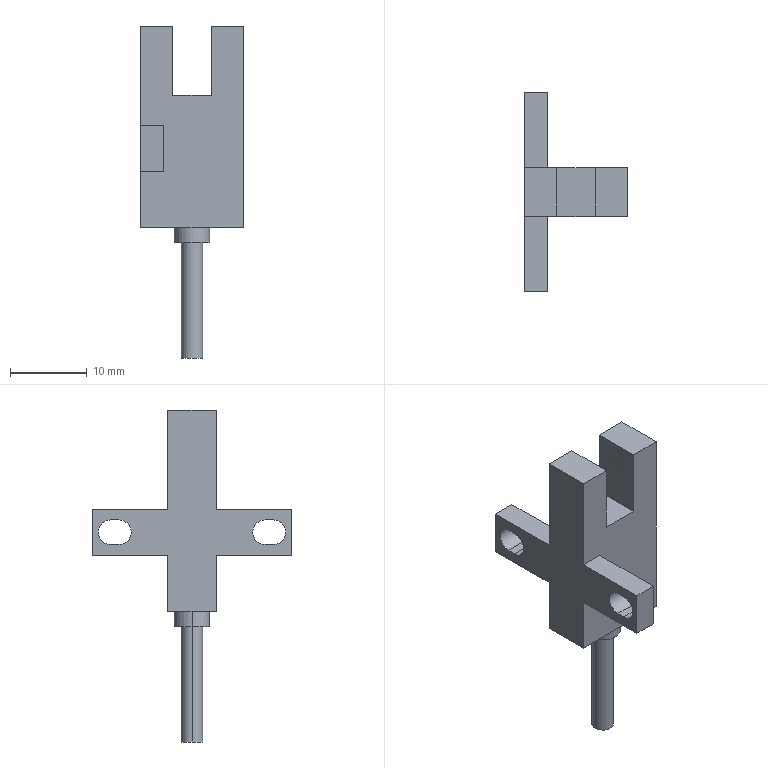Part | NX | features BREP 1 | 1 solid | 47 faces | box 13.4 x 26 x 43.2 mm | volume 2353 mm3 | plane 39 | cylinder 8 | commonest cylinder face diameters 3.2 x4 2.8 x2 4.6 x2
STEP:
#1=CARTESIAN_POINT('',(-1.4,0.,-2.));
#2=VERTEX_POINT('',#1);
#3=CARTESIAN_POINT('',(1.4,0.,-2.));
#4=VERTEX_POINT('',#3);
#5=CARTESIAN_POINT('',(0.,0.,-2.));
#6=DIRECTION('',(0.,0.,-1.));
#7=DIRECTION('',(-1.,0.,0.));
#8=AXIS2_PLACEMENT_3D('',#5,#6,#7);
#9=CIRCLE('',#8,1.4);
#10=EDGE_CURVE('',#2,#4,#9,.T.);
#11=ORIENTED_EDGE('',*,*,#10,.F.);
#12=CARTESIAN_POINT('',(0.,0.,-2.));
#13=DIRECTION('',(0.,0.,-1.));
#14=DIRECTION('',(-1.,0.,0.));
#15=AXIS2_PLACEMENT_3D('',#12,#13,#14);
#16=CIRCLE('',#15,1.4);
#17=EDGE_CURVE('',#4,#2,#16,.T.);
#18=ORIENTED_EDGE('',*,*,#17,.F.);
#19=EDGE_LOOP('',(#11,#18));
#20=FACE_BOUND('',#19,.T.);
#21=CARTESIAN_POINT('',(-2.3,0.,-2.));
#22=VERTEX_POINT('',#21);
#23=CARTESIAN_POINT('',(2.3,0.,-2.));
#24=VERTEX_POINT('',#23);
#25=CARTESIAN_POINT('',(0.,0.,-2.));
#26=DIRECTION('',(0.,0.,-1.));
#27=DIRECTION('',(-1.,0.,0.));
#28=AXIS2_PLACEMENT_3D('',#25,#26,#27);
#29=CIRCLE('',#28,2.3);
#30=EDGE_CURVE('',#22,#24,#29,.T.);
#31=ORIENTED_EDGE('',*,*,#30,.T.);
#32=CARTESIAN_POINT('',(0.,0.,-2.));
#33=DIRECTION('',(0.,0.,-1.));
#34=DIRECTION('',(-1.,0.,0.));
#35=AXIS2_PLACEMENT_3D('',#32,#33,#34);
#36=CIRCLE('',#35,2.3);
#37=EDGE_CURVE('',#24,#22,#36,.T.);
#38=ORIENTED_EDGE('',*,*,#37,.T.);
#39=EDGE_LOOP('',(#31,#38));
#40=FACE_BOUND('',#39,.T.);
#41=CARTESIAN_POINT('',(1.4,0.,-2.));
#42=DIRECTION('',(0.,0.,-1.));
#43=DIRECTION('',(-1.,0.,0.));
#44=AXIS2_PLACEMENT_3D('',#41,#42,#43);
#45=PLANE('',#44);
#46=ADVANCED_FACE('',(#20,#40),#45,.T.);
#47=CARTESIAN_POINT('',(1.4,0.,-17.));
#48=VERTEX_POINT('',#47);
#49=CARTESIAN_POINT('',(1.4,0.,0.));
#50=DIRECTION('',(0.,0.,-1.));
#51=VECTOR('',#50,1000.);
#52=LINE('',#49,#51);
#53=EDGE_CURVE('',#4,#48,#52,.T.);
#54=ORIENTED_EDGE('',*,*,#53,.F.);
#55=ORIENTED_EDGE('',*,*,#17,.T.);
#56=CARTESIAN_POINT('',(-1.4,0.,-17.));
#57=VERTEX_POINT('',#56);
#58=CARTESIAN_POINT('',(-1.4,0.,0.));
#59=DIRECTION('',(0.,0.,-1.));
#60=VECTOR('',#59,1000.);
#61=LINE('',#58,#60);
#62=EDGE_CURVE('',#2,#57,#61,.T.);
#63=ORIENTED_EDGE('',*,*,#62,.T.);
#64=CARTESIAN_POINT('',(0.,0.,-17.));
#65=DIRECTION('',(0.,0.,-1.));
#66=DIRECTION('',(-1.,0.,0.));
#67=AXIS2_PLACEMENT_3D('',#64,#65,#66);
#68=CIRCLE('',#67,1.4);
#69=EDGE_CURVE('',#48,#57,#68,.T.);
#70=ORIENTED_EDGE('',*,*,#69,.F.);
#71=EDGE_LOOP('',(#54,#55,#63,#70));
#72=FACE_BOUND('',#71,.T.);
#73=CARTESIAN_POINT('',(0.,0.,0.));
#74=DIRECTION('',(0.,0.,-1.));
#75=DIRECTION('',(-1.,0.,0.));
#76=AXIS2_PLACEMENT_3D('',#73,#74,#75);
#77=CYLINDRICAL_SURFACE('',#76,1.4);
#78=ADVANCED_FACE('',(#72),#77,.T.);
#79=CARTESIAN_POINT('',(0.,0.,-17.));
#80=DIRECTION('',(0.,0.,-1.));
#81=DIRECTION('',(-1.,0.,0.));
#82=AXIS2_PLACEMENT_3D('',#79,#80,#81);
#83=CIRCLE('',#82,1.4);
#84=EDGE_CURVE('',#57,#48,#83,.T.);
#85=ORIENTED_EDGE('',*,*,#84,.T.);
#86=ORIENTED_EDGE('',*,*,#69,.T.);
#87=EDGE_LOOP('',(#85,#86));
#88=FACE_BOUND('',#87,.T.);
#89=CARTESIAN_POINT('',(0.,0.,-17.));
#90=DIRECTION('',(0.,0.,-1.));
#91=DIRECTION('',(-1.,0.,0.));
#92=AXIS2_PLACEMENT_3D('',#89,#90,#91);
#93=PLANE('',#92);
#94=ADVANCED_FACE('',(#88),#93,.T.);
#95=CARTESIAN_POINT('',(2.3,0.,0.));
#96=VERTEX_POINT('',#95);
#97=CARTESIAN_POINT('',(2.3,0.,0.));
#98=DIRECTION('',(0.,0.,-1.));
#99=VECTOR('',#98,1000.);
#100=LINE('',#97,#99);
#101=EDGE_CURVE('',#96,#24,#100,.T.);
#102=ORIENTED_EDGE('',*,*,#101,.F.);
#103=CARTESIAN_POINT('',(-2.3,0.,0.));
#104=VERTEX_POINT('',#103);
#105=CARTESIAN_POINT('',(0.,0.,0.));
#106=DIRECTION('',(0.,0.,-1.));
#107=DIRECTION('',(-1.,0.,0.));
#108=AXIS2_PLACEMENT_3D('',#105,#106,#107);
#109=CIRCLE('',#108,2.3);
#110=EDGE_CURVE('',#96,#104,#109,.T.);
#111=ORIENTED_EDGE('',*,*,#110,.T.);
#112=CARTESIAN_POINT('',(-2.3,0.,0.));
#113=DIRECTION('',(0.,0.,-1.));
#114=VECTOR('',#113,1000.);
#115=LINE('',#112,#114);
#116=EDGE_CURVE('',#104,#22,#115,.T.);
#117=ORIENTED_EDGE('',*,*,#116,.T.);
#118=ORIENTED_EDGE('',*,*,#37,.F.);
#119=EDGE_LOOP('',(#102,#111,#117,#118));
#120=FACE_BOUND('',#119,.T.);
#121=CARTESIAN_POINT('',(0.,0.,0.));
#122=DIRECTION('',(0.,0.,-1.));
#123=DIRECTION('',(-1.,0.,0.));
#124=AXIS2_PLACEMENT_3D('',#121,#122,#123);
#125=CYLINDRICAL_SURFACE('',#124,2.3);
#126=ADVANCED_FACE('',(#120),#125,.T.);
#127=CARTESIAN_POINT('',(2.55,-0.4,22.3));
#128=VERTEX_POINT('',#127);
#129=CARTESIAN_POINT('',(2.55,-0.4,24.3));
#130=VERTEX_POINT('',#129);
#131=CARTESIAN_POINT('',(2.55,-0.4,22.3));
#132=DIRECTION('',(0.,0.,1.));
#133=VECTOR('',#132,1000.);
#134=LINE('',#131,#133);
#135=EDGE_CURVE('',#128,#130,#134,.T.);
#136=ORIENTED_EDGE('',*,*,#135,.T.);
#137=CARTESIAN_POINT('',(2.55,0.4,24.3));
#138=VERTEX_POINT('',#137);
#139=CARTESIAN_POINT('',(2.55,-0.4,24.3));
#140=DIRECTION('',(0.,1.,0.));
#141=VECTOR('',#140,1000.);
#142=LINE('',#139,#141);
#143=EDGE_CURVE('',#130,#138,#142,.T.);
#144=ORIENTED_EDGE('',*,*,#143,.T.);
#145=CARTESIAN_POINT('',(2.55,0.4,22.3));
#146=VERTEX_POINT('',#145);
#147=CARTESIAN_POINT('',(2.55,0.4,24.3));
#148=DIRECTION('',(0.,0.,-1.));
#149=VECTOR('',#148,1000.);
#150=LINE('',#147,#149);
#151=EDGE_CURVE('',#138,#146,#150,.T.);
#152=ORIENTED_EDGE('',*,*,#151,.T.);
#153=CARTESIAN_POINT('',(2.55,0.4,22.3));
#154=DIRECTION('',(0.,-1.,0.));
#155=VECTOR('',#154,1000.);
#156=LINE('',#153,#155);
#157=EDGE_CURVE('',#146,#128,#156,.T.);
#158=ORIENTED_EDGE('',*,*,#157,.T.);
#159=EDGE_LOOP('',(#136,#144,#152,#158));
#160=FACE_BOUND('',#159,.T.);
#161=CARTESIAN_POINT('',(2.55,0.,0.));
#162=DIRECTION('',(-1.,0.,0.));
#163=DIRECTION('',(0.,0.,1.));
#164=AXIS2_PLACEMENT_3D('',#161,#162,#163);
#165=PLANE('',#164);
#166=ADVANCED_FACE('',(#160),#165,.T.);
#167=CARTESIAN_POINT('',(2.5,-0.4,24.3));
#168=VERTEX_POINT('',#167);
#169=CARTESIAN_POINT('',(2.5,0.4,24.3));
#170=VERTEX_POINT('',#169);
#171=CARTESIAN_POINT('',(2.5,-0.4,24.3));
#172=DIRECTION('',(0.,1.,0.));
#173=VECTOR('',#172,1000.);
#174=LINE('',#171,#173);
#175=EDGE_CURVE('',#168,#170,#174,.T.);
#176=ORIENTED_EDGE('',*,*,#175,.T.);
#177=CARTESIAN_POINT('',(2.55,0.4,24.3));
#178=DIRECTION('',(-1.,0.,0.));
#179=VECTOR('',#178,1000.);
#180=LINE('',#177,#179);
#181=EDGE_CURVE('',#138,#170,#180,.T.);
#182=ORIENTED_EDGE('',*,*,#181,.F.);
#183=ORIENTED_EDGE('',*,*,#143,.F.);
#184=CARTESIAN_POINT('',(2.55,-0.4,24.3));
#185=DIRECTION('',(-1.,0.,0.));
#186=VECTOR('',#185,1000.);
#187=LINE('',#184,#186);
#188=EDGE_CURVE('',#130,#168,#187,.T.);
#189=ORIENTED_EDGE('',*,*,#188,.T.);
#190=EDGE_LOOP('',(#176,#182,#183,#189));
#191=FACE_BOUND('',#190,.T.);
#192=CARTESIAN_POINT('',(2.55,-0.4,24.3));
#193=DIRECTION('',(0.,0.,1.));
#194=DIRECTION('',(1.,0.,0.));
#195=AXIS2_PLACEMENT_3D('',#192,#193,#194);
#196=PLANE('',#195);
#197=ADVANCED_FACE('',(#191),#196,.F.);
#198=CARTESIAN_POINT('',(2.5,0.4,22.3));
#199=VERTEX_POINT('',#198);
#200=CARTESIAN_POINT('',(2.5,0.4,24.3));
#201=DIRECTION('',(0.,0.,-1.));
#202=VECTOR('',#201,1000.);
#203=LINE('',#200,#202);
#204=EDGE_CURVE('',#170,#199,#203,.T.);
#205=ORIENTED_EDGE('',*,*,#204,.T.);
#206=CARTESIAN_POINT('',(2.55,0.4,22.3));
#207=DIRECTION('',(-1.,0.,0.));
#208=VECTOR('',#207,1000.);
#209=LINE('',#206,#208);
#210=EDGE_CURVE('',#146,#199,#209,.T.);
#211=ORIENTED_EDGE('',*,*,#210,.F.);
#212=ORIENTED_EDGE('',*,*,#151,.F.);
#213=ORIENTED_EDGE('',*,*,#181,.T.);
#214=EDGE_LOOP('',(#205,#211,#212,#213));
#215=FACE_BOUND('',#214,.T.);
#216=CARTESIAN_POINT('',(2.55,0.4,24.3));
#217=DIRECTION('',(0.,1.,0.));
#218=DIRECTION('',(0.,0.,1.));
#219=AXIS2_PLACEMENT_3D('',#216,#217,#218);
#220=PLANE('',#219);
#221=ADVANCED_FACE('',(#215),#220,.F.);
#222=CARTESIAN_POINT('',(2.5,-0.4,22.3));
#223=VERTEX_POINT('',#222);
#224=CARTESIAN_POINT('',(2.5,0.4,22.3));
#225=DIRECTION('',(0.,-1.,0.));
#226=VECTOR('',#225,1000.);
#227=LINE('',#224,#226);
#228=EDGE_CURVE('',#199,#223,#227,.T.);
#229=ORIENTED_EDGE('',*,*,#228,.T.);
#230=CARTESIAN_POINT('',(2.55,-0.4,22.3));
#231=DIRECTION('',(-1.,0.,0.));
#232=VECTOR('',#231,1000.);
#233=LINE('',#230,#232);
#234=EDGE_CURVE('',#128,#223,#233,.T.);
#235=ORIENTED_EDGE('',*,*,#234,.F.);
#236=ORIENTED_EDGE('',*,*,#157,.F.);
#237=ORIENTED_EDGE('',*,*,#210,.T.);
#238=EDGE_LOOP('',(#229,#235,#236,#237));
#239=FACE_BOUND('',#238,.T.);
#240=CARTESIAN_POINT('',(2.55,0.4,22.3));
#241=DIRECTION('',(0.,0.,-1.));
#242=DIRECTION('',(-1.,0.,0.));
#243=AXIS2_PLACEMENT_3D('',#240,#241,#242);
#244=PLANE('',#243);
#245=ADVANCED_FACE('',(#239),#244,.F.);
#246=CARTESIAN_POINT('',(2.5,-0.4,22.3));
#247=DIRECTION('',(0.,0.,1.));
#248=VECTOR('',#247,1000.);
#249=LINE('',#246,#248);
#250=EDGE_CURVE('',#223,#168,#249,.T.);
#251=ORIENTED_EDGE('',*,*,#250,.T.);
#252=ORIENTED_EDGE('',*,*,#188,.F.);
#253=ORIENTED_EDGE('',*,*,#135,.F.);
#254=ORIENTED_EDGE('',*,*,#234,.T.);
#255=EDGE_LOOP('',(#251,#252,#253,#254));
#256=FACE_BOUND('',#255,.T.);
#257=CARTESIAN_POINT('',(2.55,-0.4,22.3));
#258=DIRECTION('',(0.,-1.,0.));
#259=DIRECTION('',(0.,0.,-1.));
#260=AXIS2_PLACEMENT_3D('',#257,#258,#259);
#261=PLANE('',#260);
#262=ADVANCED_FACE('',(#256),#261,.F.);
#263=CARTESIAN_POINT('',(-2.55,-0.4,22.3));
#264=VERTEX_POINT('',#263);
#265=CARTESIAN_POINT('',(-2.55,0.4,22.3));
#266=VERTEX_POINT('',#265);
#267=CARTESIAN_POINT('',(-2.55,-0.4,22.3));
#268=DIRECTION('',(0.,1.,0.));
#269=VECTOR('',#268,1000.);
#270=LINE('',#267,#269);
#271=EDGE_CURVE('',#264,#266,#270,.T.);
#272=ORIENTED_EDGE('',*,*,#271,.T.);
#273=CARTESIAN_POINT('',(-2.55,0.4,24.3));
#274=VERTEX_POINT('',#273);
#275=CARTESIAN_POINT('',(-2.55,0.4,22.3));
#276=DIRECTION('',(0.,0.,1.));
#277=VECTOR('',#276,1000.);
#278=LINE('',#275,#277);
#279=EDGE_CURVE('',#266,#274,#278,.T.);
#280=ORIENTED_EDGE('',*,*,#279,.T.);
#281=CARTESIAN_POINT('',(-2.55,-0.4,24.3));
#282=VERTEX_POINT('',#281);
#283=CARTESIAN_POINT('',(-2.55,0.4,24.3));
#284=DIRECTION('',(0.,-1.,0.));
#285=VECTOR('',#284,1000.);
#286=LINE('',#283,#285);
#287=EDGE_CURVE('',#274,#282,#286,.T.);
#288=ORIENTED_EDGE('',*,*,#287,.T.);
#289=CARTESIAN_POINT('',(-2.55,-0.4,24.3));
#290=DIRECTION('',(0.,0.,-1.));
#291=VECTOR('',#290,1000.);
#292=LINE('',#289,#291);
#293=EDGE_CURVE('',#282,#264,#292,.T.);
#294=ORIENTED_EDGE('',*,*,#293,.T.);
#295=EDGE_LOOP('',(#272,#280,#288,#294));
#296=FACE_BOUND('',#295,.T.);
#297=CARTESIAN_POINT('',(-2.55,0.,0.));
#298=DIRECTION('',(1.,0.,0.));
#299=DIRECTION('',(0.,0.,-1.));
#300=AXIS2_PLACEMENT_3D('',#297,#298,#299);
#301=PLANE('',#300);
#302=ADVANCED_FACE('',(#296),#301,.T.);
#303=CARTESIAN_POINT('',(-2.5,0.4,22.3));
#304=VERTEX_POINT('',#303);
#305=CARTESIAN_POINT('',(-2.5,0.4,24.3));
#306=VERTEX_POINT('',#305);
#307=CARTESIAN_POINT('',(-2.5,0.4,22.3));
#308=DIRECTION('',(0.,0.,1.));
#309=VECTOR('',#308,1000.);
#310=LINE('',#307,#309);
#311=EDGE_CURVE('',#304,#306,#310,.T.);
#312=ORIENTED_EDGE('',*,*,#311,.T.);
#313=CARTESIAN_POINT('',(-2.55,0.4,24.3));
#314=DIRECTION('',(1.,0.,0.));
#315=VECTOR('',#314,1000.);
#316=LINE('',#313,#315);
#317=EDGE_CURVE('',#274,#306,#316,.T.);
#318=ORIENTED_EDGE('',*,*,#317,.F.);
#319=ORIENTED_EDGE('',*,*,#279,.F.);
#320=CARTESIAN_POINT('',(-2.55,0.4,22.3));
#321=DIRECTION('',(1.,0.,0.));
#322=VECTOR('',#321,1000.);
#323=LINE('',#320,#322);
#324=EDGE_CURVE('',#266,#304,#323,.T.);
#325=ORIENTED_EDGE('',*,*,#324,.T.);
#326=EDGE_LOOP('',(#312,#318,#319,#325));
#327=FACE_BOUND('',#326,.T.);
#328=CARTESIAN_POINT('',(-2.55,0.4,22.3));
#329=DIRECTION('',(0.,1.,0.));
#330=DIRECTION('',(0.,0.,1.));
#331=AXIS2_PLACEMENT_3D('',#328,#329,#330);
#332=PLANE('',#331);
#333=ADVANCED_FACE('',(#327),#332,.F.);
#334=CARTESIAN_POINT('',(-2.5,-0.4,24.3));
#335=VERTEX_POINT('',#334);
#336=CARTESIAN_POINT('',(-2.5,0.4,24.3));
#337=DIRECTION('',(0.,-1.,0.));
#338=VECTOR('',#337,1000.);
#339=LINE('',#336,#338);
#340=EDGE_CURVE('',#306,#335,#339,.T.);
#341=ORIENTED_EDGE('',*,*,#340,.T.);
#342=CARTESIAN_POINT('',(-2.55,-0.4,24.3));
#343=DIRECTION('',(1.,0.,0.));
#344=VECTOR('',#343,1000.);
#345=LINE('',#342,#344);
#346=EDGE_CURVE('',#282,#335,#345,.T.);
#347=ORIENTED_EDGE('',*,*,#346,.F.);
#348=ORIENTED_EDGE('',*,*,#287,.F.);
#349=ORIENTED_EDGE('',*,*,#317,.T.);
#350=EDGE_LOOP('',(#341,#347,#348,#349));
#351=FACE_BOUND('',#350,.T.);
#352=CARTESIAN_POINT('',(-2.55,0.4,24.3));
#353=DIRECTION('',(0.,0.,1.));
#354=DIRECTION('',(1.,0.,0.));
#355=AXIS2_PLACEMENT_3D('',#352,#353,#354);
#356=PLANE('',#355);
#357=ADVANCED_FACE('',(#351),#356,.F.);
#358=CARTESIAN_POINT('',(-2.5,-0.4,22.3));
#359=VERTEX_POINT('',#358);
#360=CARTESIAN_POINT('',(-2.5,-0.4,24.3));
#361=DIRECTION('',(0.,0.,-1.));
#362=VECTOR('',#361,1000.);
#363=LINE('',#360,#362);
#364=EDGE_CURVE('',#335,#359,#363,.T.);
#365=ORIENTED_EDGE('',*,*,#364,.T.);
#366=CARTESIAN_POINT('',(-2.55,-0.4,22.3));
#367=DIRECTION('',(1.,0.,0.));
#368=VECTOR('',#367,1000.);
#369=LINE('',#366,#368);
#370=EDGE_CURVE('',#264,#359,#369,.T.);
#371=ORIENTED_EDGE('',*,*,#370,.F.);
#372=ORIENTED_EDGE('',*,*,#293,.F.);
#373=ORIENTED_EDGE('',*,*,#346,.T.);
#374=EDGE_LOOP('',(#365,#371,#372,#373));
#375=FACE_BOUND('',#374,.T.);
#376=CARTESIAN_POINT('',(-2.55,-0.4,24.3));
#377=DIRECTION('',(0.,-1.,0.));
#378=DIRECTION('',(0.,0.,-1.));
#379=AXIS2_PLACEMENT_3D('',#376,#377,#378);
#380=PLANE('',#379);
#381=ADVANCED_FACE('',(#375),#380,.F.);
#382=CARTESIAN_POINT('',(-2.5,-0.4,22.3));
#383=DIRECTION('',(0.,1.,0.));
#384=VECTOR('',#383,1000.);
#385=LINE('',#382,#384);
#386=EDGE_CURVE('',#359,#304,#385,.T.);
#387=ORIENTED_EDGE('',*,*,#386,.T.);
#388=ORIENTED_EDGE('',*,*,#324,.F.);
#389=ORIENTED_EDGE('',*,*,#271,.F.);
#390=ORIENTED_EDGE('',*,*,#370,.T.);
#391=EDGE_LOOP('',(#387,#388,#389,#390));
#392=FACE_BOUND('',#391,.T.);
#393=CARTESIAN_POINT('',(-2.55,-0.4,22.3));
#394=DIRECTION('',(0.,0.,-1.));
#395=DIRECTION('',(-1.,0.,0.));
#396=AXIS2_PLACEMENT_3D('',#393,#394,#395);
#397=PLANE('',#396);
#398=ADVANCED_FACE('',(#392),#397,.F.);
#399=CARTESIAN_POINT('',(3.,3.125,11.3));
#400=VERTEX_POINT('',#399);
#401=CARTESIAN_POINT('',(3.,3.125,8.8));
#402=VERTEX_POINT('',#401);
#403=CARTESIAN_POINT('',(3.,3.125,11.3));
#404=DIRECTION('',(0.,0.,-1.));
#405=VECTOR('',#404,1000.);
#406=LINE('',#403,#405);
#407=EDGE_CURVE('',#400,#402,#406,.T.);
#408=ORIENTED_EDGE('',*,*,#407,.T.);
#409=CARTESIAN_POINT('',(0.,3.125,8.8));
#410=VERTEX_POINT('',#409);
#411=CARTESIAN_POINT('',(3.,3.125,8.8));
#412=DIRECTION('',(-1.,0.,0.));
#413=VECTOR('',#412,1000.);
#414=LINE('',#411,#413);
#415=EDGE_CURVE('',#402,#410,#414,.T.);
#416=ORIENTED_EDGE('',*,*,#415,.T.);
#417=CARTESIAN_POINT('',(0.,3.125,11.3));
#418=VERTEX_POINT('',#417);
#419=CARTESIAN_POINT('',(0.,3.125,8.8));
#420=DIRECTION('',(0.,0.,1.));
#421=VECTOR('',#420,1000.);
#422=LINE('',#419,#421);
#423=EDGE_CURVE('',#410,#418,#422,.T.);
#424=ORIENTED_EDGE('',*,*,#423,.T.);
#425=CARTESIAN_POINT('',(0.,3.125,11.3));
#426=DIRECTION('',(1.,0.,0.));
#427=VECTOR('',#426,1000.);
#428=LINE('',#425,#427);
#429=EDGE_CURVE('',#418,#400,#428,.T.);
#430=ORIENTED_EDGE('',*,*,#429,.T.);
#431=EDGE_LOOP('',(#408,#416,#424,#430));
#432=FACE_BOUND('',#431,.T.);
#433=CARTESIAN_POINT('',(0.,3.125,0.));
#434=DIRECTION('',(0.,1.,0.));
#435=DIRECTION('',(0.,0.,1.));
#436=AXIS2_PLACEMENT_3D('',#433,#434,#435);
#437=PLANE('',#436);
#438=ADVANCED_FACE('',(#432),#437,.T.);
#439=CARTESIAN_POINT('',(3.,3.175,8.8));
#440=VERTEX_POINT('',#439);
#441=CARTESIAN_POINT('',(0.,3.175,8.8));
#442=VERTEX_POINT('',#441);
#443=CARTESIAN_POINT('',(3.,3.175,8.8));
#444=DIRECTION('',(-1.,0.,0.));
#445=VECTOR('',#444,1000.);
#446=LINE('',#443,#445);
#447=EDGE_CURVE('',#440,#442,#446,.T.);
#448=ORIENTED_EDGE('',*,*,#447,.T.);
#449=CARTESIAN_POINT('',(0.,3.125,8.8));
#450=DIRECTION('',(0.,1.,0.));
#451=VECTOR('',#450,1000.);
#452=LINE('',#449,#451);
#453=EDGE_CURVE('',#410,#442,#452,.T.);
#454=ORIENTED_EDGE('',*,*,#453,.F.);
#455=ORIENTED_EDGE('',*,*,#415,.F.);
#456=CARTESIAN_POINT('',(3.,3.125,8.8));
#457=DIRECTION('',(0.,1.,0.));
#458=VECTOR('',#457,1000.);
#459=LINE('',#456,#458);
#460=EDGE_CURVE('',#402,#440,#459,.T.);
#461=ORIENTED_EDGE('',*,*,#460,.T.);
#462=EDGE_LOOP('',(#448,#454,#455,#461));
#463=FACE_BOUND('',#462,.T.);
#464=CARTESIAN_POINT('',(3.,3.125,8.8));
#465=DIRECTION('',(0.,0.,-1.));
#466=DIRECTION('',(-1.,0.,0.));
#467=AXIS2_PLACEMENT_3D('',#464,#465,#466);
#468=PLANE('',#467);
#469=ADVANCED_FACE('',(#463),#468,.F.);
#470=CARTESIAN_POINT('',(0.,3.175,11.3));
#471=VERTEX_POINT('',#470);
#472=CARTESIAN_POINT('',(0.,3.175,8.8));
#473=DIRECTION('',(0.,0.,1.));
#474=VECTOR('',#473,1000.);
#475=LINE('',#472,#474);
#476=EDGE_CURVE('',#442,#471,#475,.T.);
#477=ORIENTED_EDGE('',*,*,#476,.T.);
#478=CARTESIAN_POINT('',(0.,3.125,11.3));
#479=DIRECTION('',(0.,1.,0.));
#480=VECTOR('',#479,1000.);
#481=LINE('',#478,#480);
#482=EDGE_CURVE('',#418,#471,#481,.T.);
#483=ORIENTED_EDGE('',*,*,#482,.F.);
#484=ORIENTED_EDGE('',*,*,#423,.F.);
#485=ORIENTED_EDGE('',*,*,#453,.T.);
#486=EDGE_LOOP('',(#477,#483,#484,#485));
#487=FACE_BOUND('',#486,.T.);
#488=CARTESIAN_POINT('',(0.,3.125,8.8));
#489=DIRECTION('',(-1.,0.,0.));
#490=DIRECTION('',(0.,0.,1.));
#491=AXIS2_PLACEMENT_3D('',#488,#489,#490);
#492=PLANE('',#491);
#493=ADVANCED_FACE('',(#487),#492,.F.);
#494=CARTESIAN_POINT('',(3.,3.175,11.3));
#495=VERTEX_POINT('',#494);
#496=CARTESIAN_POINT('',(0.,3.175,11.3));
#497=DIRECTION('',(1.,0.,0.));
#498=VECTOR('',#497,1000.);
#499=LINE('',#496,#498);
#500=EDGE_CURVE('',#471,#495,#499,.T.);
#501=ORIENTED_EDGE('',*,*,#500,.T.);
#502=CARTESIAN_POINT('',(3.,3.125,11.3));
#503=DIRECTION('',(0.,1.,0.));
#504=VECTOR('',#503,1000.);
#505=LINE('',#502,#504);
#506=EDGE_CURVE('',#400,#495,#505,.T.);
#507=ORIENTED_EDGE('',*,*,#506,.F.);
#508=ORIENTED_EDGE('',*,*,#429,.F.);
#509=ORIENTED_EDGE('',*,*,#482,.T.);
#510=EDGE_LOOP('',(#501,#507,#508,#509));
#511=FACE_BOUND('',#510,.T.);
#512=CARTESIAN_POINT('',(0.,3.125,11.3));
#513=DIRECTION('',(0.,0.,1.));
#514=DIRECTION('',(1.,0.,0.));
#515=AXIS2_PLACEMENT_3D('',#512,#513,#514);
#516=PLANE('',#515);
#517=ADVANCED_FACE('',(#511),#516,.F.);
#518=CARTESIAN_POINT('',(3.,3.175,11.3));
#519=DIRECTION('',(0.,0.,-1.));
#520=VECTOR('',#519,1000.);
#521=LINE('',#518,#520);
#522=EDGE_CURVE('',#495,#440,#521,.T.);
#523=ORIENTED_EDGE('',*,*,#522,.T.);
#524=ORIENTED_EDGE('',*,*,#460,.F.);
#525=ORIENTED_EDGE('',*,*,#407,.F.);
#526=ORIENTED_EDGE('',*,*,#506,.T.);
#527=EDGE_LOOP('',(#523,#524,#525,#526));
#528=FACE_BOUND('',#527,.T.);
#529=CARTESIAN_POINT('',(3.,3.125,11.3));
#530=DIRECTION('',(1.,0.,0.));
#531=DIRECTION('',(0.,0.,-1.));
#532=AXIS2_PLACEMENT_3D('',#529,#530,#531);
#533=PLANE('',#532);
#534=ADVANCED_FACE('',(#528),#533,.F.);
#535=CARTESIAN_POINT('',(-3.7,9.5,11.9));
#536=VERTEX_POINT('',#535);
#537=CARTESIAN_POINT('',(-6.7,9.5,11.9));
#538=VERTEX_POINT('',#537);
#539=CARTESIAN_POINT('',(6.7,9.5,11.9));
#540=DIRECTION('',(-1.,0.,0.));
#541=VECTOR('',#540,1000.);
#542=LINE('',#539,#541);
#543=EDGE_CURVE('',#536,#538,#542,.T.);
#544=ORIENTED_EDGE('',*,*,#543,.T.);
#545=CARTESIAN_POINT('',(-6.7,10.6,11.9));
#546=VERTEX_POINT('',#545);
#547=CARTESIAN_POINT('',(-6.7,9.5,11.9));
#548=DIRECTION('',(0.,1.,0.));
#549=VECTOR('',#548,1000.);
#550=LINE('',#547,#549);
#551=EDGE_CURVE('',#538,#546,#550,.T.);
#552=ORIENTED_EDGE('',*,*,#551,.T.);
#553=CARTESIAN_POINT('',(-3.7,10.6,11.9));
#554=VERTEX_POINT('',#553);
#555=CARTESIAN_POINT('',(6.7,10.6,11.9));
#556=DIRECTION('',(-1.,0.,0.));
#557=VECTOR('',#556,1000.);
#558=LINE('',#555,#557);
#559=EDGE_CURVE('',#554,#546,#558,.T.);
#560=ORIENTED_EDGE('',*,*,#559,.F.);
#561=CARTESIAN_POINT('',(-3.7,13.,11.9));
#562=DIRECTION('',(0.,1.,0.));
#563=VECTOR('',#562,1000.);
#564=LINE('',#561,#563);
#565=EDGE_CURVE('',#536,#554,#564,.T.);
#566=ORIENTED_EDGE('',*,*,#565,.F.);
#567=EDGE_LOOP('',(#544,#552,#560,#566));
#568=FACE_BOUND('',#567,.T.);
#569=CARTESIAN_POINT('',(6.7,9.5,11.9));
#570=DIRECTION('',(0.,0.,1.));
#571=DIRECTION('',(1.,0.,0.));
#572=AXIS2_PLACEMENT_3D('',#569,#570,#571);
#573=PLANE('',#572);
#574=ADVANCED_FACE('',(#568),#573,.F.);
#575=ORIENTED_EDGE('',*,*,#559,.T.);
#576=CARTESIAN_POINT('',(-6.7,10.6,8.7));
#577=VERTEX_POINT('',#576);
#578=CARTESIAN_POINT('',(-6.7,10.6,10.3));
#579=DIRECTION('',(-1.,0.,0.));
#580=DIRECTION('',(0.,0.,1.));
#581=AXIS2_PLACEMENT_3D('',#578,#579,#580);
#582=CIRCLE('',#581,1.6);
#583=EDGE_CURVE('',#546,#577,#582,.T.);
#584=ORIENTED_EDGE('',*,*,#583,.T.);
#585=CARTESIAN_POINT('',(-3.7,10.6,8.7));
#586=VERTEX_POINT('',#585);
#587=CARTESIAN_POINT('',(6.7,10.6,8.7));
#588=DIRECTION('',(-1.,0.,0.));
#589=VECTOR('',#588,1000.);
#590=LINE('',#587,#589);
#591=EDGE_CURVE('',#586,#577,#590,.T.);
#592=ORIENTED_EDGE('',*,*,#591,.F.);
#593=CARTESIAN_POINT('',(-3.7,10.6,10.3));
#594=DIRECTION('',(-1.,0.,0.));
#595=DIRECTION('',(0.,0.,1.));
#596=AXIS2_PLACEMENT_3D('',#593,#594,#595);
#597=CIRCLE('',#596,1.6);
#598=EDGE_CURVE('',#554,#586,#597,.T.);
#599=ORIENTED_EDGE('',*,*,#598,.F.);
#600=EDGE_LOOP('',(#575,#584,#592,#599));
#601=FACE_BOUND('',#600,.T.);
#602=CARTESIAN_POINT('',(6.7,10.6,10.3));
#603=DIRECTION('',(-1.,0.,0.));
#604=DIRECTION('',(0.,0.,1.));
#605=AXIS2_PLACEMENT_3D('',#602,#603,#604);
#606=CYLINDRICAL_SURFACE('',#605,1.6);
#607=ADVANCED_FACE('',(#601),#606,.F.);
#608=ORIENTED_EDGE('',*,*,#591,.T.);
#609=CARTESIAN_POINT('',(-6.7,9.5,8.7));
#610=VERTEX_POINT('',#609);
#611=CARTESIAN_POINT('',(-6.7,10.6,8.7));
#612=DIRECTION('',(0.,-1.,0.));
#613=VECTOR('',#612,1000.);
#614=LINE('',#611,#613);
#615=EDGE_CURVE('',#577,#610,#614,.T.);
#616=ORIENTED_EDGE('',*,*,#615,.T.);
#617=CARTESIAN_POINT('',(-3.7,9.5,8.7));
#618=VERTEX_POINT('',#617);
#619=CARTESIAN_POINT('',(6.7,9.5,8.7));
#620=DIRECTION('',(-1.,0.,0.));
#621=VECTOR('',#620,1000.);
#622=LINE('',#619,#621);
#623=EDGE_CURVE('',#618,#610,#622,.T.);
#624=ORIENTED_EDGE('',*,*,#623,.F.);
#625=CARTESIAN_POINT('',(-3.7,13.,8.7));
#626=DIRECTION('',(0.,-1.,0.));
#627=VECTOR('',#626,1000.);
#628=LINE('',#625,#627);
#629=EDGE_CURVE('',#586,#618,#628,.T.);
#630=ORIENTED_EDGE('',*,*,#629,.F.);
#631=EDGE_LOOP('',(#608,#616,#624,#630));
#632=FACE_BOUND('',#631,.T.);
#633=CARTESIAN_POINT('',(6.7,10.6,8.7));
#634=DIRECTION('',(0.,0.,-1.));
#635=DIRECTION('',(-1.,0.,0.));
#636=AXIS2_PLACEMENT_3D('',#633,#634,#635);
#637=PLANE('',#636);
#638=ADVANCED_FACE('',(#632),#637,.F.);
#639=ORIENTED_EDGE('',*,*,#623,.T.);
#640=CARTESIAN_POINT('',(-6.7,9.5,10.3));
#641=DIRECTION('',(-1.,0.,0.));
#642=DIRECTION('',(0.,0.,1.));
#643=AXIS2_PLACEMENT_3D('',#640,#641,#642);
#644=CIRCLE('',#643,1.6);
#645=EDGE_CURVE('',#610,#538,#644,.T.);
#646=ORIENTED_EDGE('',*,*,#645,.T.);
#647=ORIENTED_EDGE('',*,*,#543,.F.);
#648=CARTESIAN_POINT('',(-3.7,9.5,10.3));
#649=DIRECTION('',(-1.,0.,0.));
#650=DIRECTION('',(0.,0.,1.));
#651=AXIS2_PLACEMENT_3D('',#648,#649,#650);
#652=CIRCLE('',#651,1.6);
#653=EDGE_CURVE('',#618,#536,#652,.T.);
#654=ORIENTED_EDGE('',*,*,#653,.F.);
#655=EDGE_LOOP('',(#639,#646,#647,#654));
#656=FACE_BOUND('',#655,.T.);
#657=CARTESIAN_POINT('',(6.7,9.5,10.3));
#658=DIRECTION('',(-1.,0.,0.));
#659=DIRECTION('',(0.,0.,1.));
#660=AXIS2_PLACEMENT_3D('',#657,#658,#659);
#661=CYLINDRICAL_SURFACE('',#660,1.6);
#662=ADVANCED_FACE('',(#656),#661,.F.);
#663=CARTESIAN_POINT('',(-6.7,13.,7.3));
#664=VERTEX_POINT('',#663);
#665=CARTESIAN_POINT('',(-6.7,13.,13.3));
#666=VERTEX_POINT('',#665);
#667=CARTESIAN_POINT('',(-6.7,13.,13.3));
#668=DIRECTION('',(0.,0.,1.));
#669=VECTOR('',#668,1000.);
#670=LINE('',#667,#669);
#671=EDGE_CURVE('',#664,#666,#670,.T.);
#672=ORIENTED_EDGE('',*,*,#671,.T.);
#673=CARTESIAN_POINT('',(-3.7,13.,13.3));
#674=VERTEX_POINT('',#673);
#675=CARTESIAN_POINT('',(-3.7,13.,13.3));
#676=DIRECTION('',(1.,0.,0.));
#677=VECTOR('',#676,1000.);
#678=LINE('',#675,#677);
#679=EDGE_CURVE('',#666,#674,#678,.T.);
#680=ORIENTED_EDGE('',*,*,#679,.T.);
#681=CARTESIAN_POINT('',(-3.7,13.,7.3));
#682=VERTEX_POINT('',#681);
#683=CARTESIAN_POINT('',(-3.7,13.,7.3));
#684=DIRECTION('',(0.,0.,-1.));
#685=VECTOR('',#684,1000.);
#686=LINE('',#683,#685);
#687=EDGE_CURVE('',#674,#682,#686,.T.);
#688=ORIENTED_EDGE('',*,*,#687,.T.);
#689=CARTESIAN_POINT('',(-6.7,13.,7.3));
#690=DIRECTION('',(-1.,0.,0.));
#691=VECTOR('',#690,1000.);
#692=LINE('',#689,#691);
#693=EDGE_CURVE('',#682,#664,#692,.T.);
#694=ORIENTED_EDGE('',*,*,#693,.T.);
#695=EDGE_LOOP('',(#672,#680,#688,#694));
#696=FACE_BOUND('',#695,.T.);
#697=CARTESIAN_POINT('',(0.,13.,0.));
#698=DIRECTION('',(0.,-1.,0.));
#699=DIRECTION('',(0.,0.,-1.));
#700=AXIS2_PLACEMENT_3D('',#697,#698,#699);
#701=PLANE('',#700);
#702=ADVANCED_FACE('',(#696),#701,.F.);
#703=CARTESIAN_POINT('',(-3.7,3.175,7.3));
#704=VERTEX_POINT('',#703);
#705=CARTESIAN_POINT('',(-6.7,3.175,7.3));
#706=VERTEX_POINT('',#705);
#707=CARTESIAN_POINT('',(-6.7,3.175,7.3));
#708=DIRECTION('',(-1.,0.,0.));
#709=VECTOR('',#708,1000.);
#710=LINE('',#707,#709);
#711=EDGE_CURVE('',#704,#706,#710,.T.);
#712=ORIENTED_EDGE('',*,*,#711,.T.);
#713=CARTESIAN_POINT('',(-6.7,13.,7.3));
#714=DIRECTION('',(0.,-1.,0.));
#715=VECTOR('',#714,1000.);
#716=LINE('',#713,#715);
#717=EDGE_CURVE('',#664,#706,#716,.T.);
#718=ORIENTED_EDGE('',*,*,#717,.F.);
#719=ORIENTED_EDGE('',*,*,#693,.F.);
#720=CARTESIAN_POINT('',(-3.7,13.,7.3));
#721=DIRECTION('',(0.,-1.,0.));
#722=VECTOR('',#721,1000.);
#723=LINE('',#720,#722);
#724=EDGE_CURVE('',#682,#704,#723,.T.);
#725=ORIENTED_EDGE('',*,*,#724,.T.);
#726=EDGE_LOOP('',(#712,#718,#719,#725));
#727=FACE_BOUND('',#726,.T.);
#728=CARTESIAN_POINT('',(-6.7,13.,7.3));
#729=DIRECTION('',(0.,0.,1.));
#730=DIRECTION('',(1.,0.,0.));
#731=AXIS2_PLACEMENT_3D('',#728,#729,#730);
#732=PLANE('',#731);
#733=ADVANCED_FACE('',(#727),#732,.F.);
#734=CARTESIAN_POINT('',(-3.7,3.175,13.3));
#735=VERTEX_POINT('',#734);
#736=CARTESIAN_POINT('',(-3.7,3.175,7.3));
#737=DIRECTION('',(0.,0.,-1.));
#738=VECTOR('',#737,1000.);
#739=LINE('',#736,#738);
#740=EDGE_CURVE('',#735,#704,#739,.T.);
#741=ORIENTED_EDGE('',*,*,#740,.T.);
#742=ORIENTED_EDGE('',*,*,#724,.F.);
#743=ORIENTED_EDGE('',*,*,#687,.F.);
#744=CARTESIAN_POINT('',(-3.7,13.,13.3));
#745=DIRECTION('',(0.,-1.,0.));
#746=VECTOR('',#745,1000.);
#747=LINE('',#744,#746);
#748=EDGE_CURVE('',#674,#735,#747,.T.);
#749=ORIENTED_EDGE('',*,*,#748,.T.);
#750=EDGE_LOOP('',(#741,#742,#743,#749));
#751=FACE_BOUND('',#750,.T.);
#752=ORIENTED_EDGE('',*,*,#629,.T.);
#753=ORIENTED_EDGE('',*,*,#653,.T.);
#754=ORIENTED_EDGE('',*,*,#565,.T.);
#755=ORIENTED_EDGE('',*,*,#598,.T.);
#756=EDGE_LOOP('',(#752,#753,#754,#755));
#757=FACE_BOUND('',#756,.T.);
#758=CARTESIAN_POINT('',(-3.7,13.,7.3));
#759=DIRECTION('',(-1.,0.,0.));
#760=DIRECTION('',(0.,0.,1.));
#761=AXIS2_PLACEMENT_3D('',#758,#759,#760);
#762=PLANE('',#761);
#763=ADVANCED_FACE('',(#751,#757),#762,.F.);
#764=CARTESIAN_POINT('',(-6.7,3.175,13.3));
#765=VERTEX_POINT('',#764);
#766=CARTESIAN_POINT('',(-3.7,3.175,13.3));
#767=DIRECTION('',(1.,0.,0.));
#768=VECTOR('',#767,1000.);
#769=LINE('',#766,#768);
#770=EDGE_CURVE('',#765,#735,#769,.T.);
#771=ORIENTED_EDGE('',*,*,#770,.T.);
#772=ORIENTED_EDGE('',*,*,#748,.F.);
#773=ORIENTED_EDGE('',*,*,#679,.F.);
#774=CARTESIAN_POINT('',(-6.7,13.,13.3));
#775=DIRECTION('',(0.,-1.,0.));
#776=VECTOR('',#775,1000.);
#777=LINE('',#774,#776);
#778=EDGE_CURVE('',#666,#765,#777,.T.);
#779=ORIENTED_EDGE('',*,*,#778,.T.);
#780=EDGE_LOOP('',(#771,#772,#773,#779));
#781=FACE_BOUND('',#780,.T.);
#782=CARTESIAN_POINT('',(-3.7,13.,13.3));
#783=DIRECTION('',(0.,0.,-1.));
#784=DIRECTION('',(-1.,0.,0.));
#785=AXIS2_PLACEMENT_3D('',#782,#783,#784);
#786=PLANE('',#785);
#787=ADVANCED_FACE('',(#781),#786,.F.);
#788=CARTESIAN_POINT('',(-3.7,-10.6,8.7));
#789=VERTEX_POINT('',#788);
#790=CARTESIAN_POINT('',(-3.7,-9.5,8.7));
#791=VERTEX_POINT('',#790);
#792=CARTESIAN_POINT('',(-3.7,-10.6,8.7));
#793=DIRECTION('',(0.,1.,0.));
#794=VECTOR('',#793,1000.);
#795=LINE('',#792,#794);
#796=EDGE_CURVE('',#789,#791,#795,.T.);
#797=ORIENTED_EDGE('',*,*,#796,.T.);
#798=CARTESIAN_POINT('',(-6.7,-9.5,8.7));
#799=VERTEX_POINT('',#798);
#800=CARTESIAN_POINT('',(-6.7,-9.5,8.7));
#801=DIRECTION('',(1.,0.,0.));
#802=VECTOR('',#801,1000.);
#803=LINE('',#800,#802);
#804=EDGE_CURVE('',#799,#791,#803,.T.);
#805=ORIENTED_EDGE('',*,*,#804,.F.);
#806=CARTESIAN_POINT('',(-6.7,-10.6,8.7));
#807=VERTEX_POINT('',#806);
#808=CARTESIAN_POINT('',(-6.7,-10.6,8.7));
#809=DIRECTION('',(0.,1.,0.));
#810=VECTOR('',#809,1000.);
#811=LINE('',#808,#810);
#812=EDGE_CURVE('',#807,#799,#811,.T.);
#813=ORIENTED_EDGE('',*,*,#812,.F.);
#814=CARTESIAN_POINT('',(-6.7,-10.6,8.7));
#815=DIRECTION('',(1.,0.,0.));
#816=VECTOR('',#815,1000.);
#817=LINE('',#814,#816);
#818=EDGE_CURVE('',#807,#789,#817,.T.);
#819=ORIENTED_EDGE('',*,*,#818,.T.);
#820=EDGE_LOOP('',(#797,#805,#813,#819));
#821=FACE_BOUND('',#820,.T.);
#822=CARTESIAN_POINT('',(-6.7,-10.6,8.7));
#823=DIRECTION('',(0.,0.,-1.));
#824=DIRECTION('',(-1.,0.,0.));
#825=AXIS2_PLACEMENT_3D('',#822,#823,#824);
#826=PLANE('',#825);
#827=ADVANCED_FACE('',(#821),#826,.F.);
#828=CARTESIAN_POINT('',(-3.7,-9.5,11.9));
#829=VERTEX_POINT('',#828);
#830=CARTESIAN_POINT('',(-3.7,-9.5,10.3));
#831=DIRECTION('',(1.,0.,0.));
#832=DIRECTION('',(0.,0.,-1.));
#833=AXIS2_PLACEMENT_3D('',#830,#831,#832);
#834=CIRCLE('',#833,1.6);
#835=EDGE_CURVE('',#791,#829,#834,.T.);
#836=ORIENTED_EDGE('',*,*,#835,.T.);
#837=CARTESIAN_POINT('',(-6.7,-9.5,11.9));
#838=VERTEX_POINT('',#837);
#839=CARTESIAN_POINT('',(-6.7,-9.5,11.9));
#840=DIRECTION('',(1.,0.,0.));
#841=VECTOR('',#840,1000.);
#842=LINE('',#839,#841);
#843=EDGE_CURVE('',#838,#829,#842,.T.);
#844=ORIENTED_EDGE('',*,*,#843,.F.);
#845=CARTESIAN_POINT('',(-6.7,-9.5,10.3));
#846=DIRECTION('',(1.,0.,0.));
#847=DIRECTION('',(0.,0.,-1.));
#848=AXIS2_PLACEMENT_3D('',#845,#846,#847);
#849=CIRCLE('',#848,1.6);
#850=EDGE_CURVE('',#799,#838,#849,.T.);
#851=ORIENTED_EDGE('',*,*,#850,.F.);
#852=ORIENTED_EDGE('',*,*,#804,.T.);
#853=EDGE_LOOP('',(#836,#844,#851,#852));
#854=FACE_BOUND('',#853,.T.);
#855=CARTESIAN_POINT('',(-6.7,-9.5,10.3));
#856=DIRECTION('',(1.,0.,0.));
#857=DIRECTION('',(0.,0.,-1.));
#858=AXIS2_PLACEMENT_3D('',#855,#856,#857);
#859=CYLINDRICAL_SURFACE('',#858,1.6);
#860=ADVANCED_FACE('',(#854),#859,.F.);
#861=CARTESIAN_POINT('',(-3.7,-10.6,11.9));
#862=VERTEX_POINT('',#861);
#863=CARTESIAN_POINT('',(-3.7,-9.5,11.9));
#864=DIRECTION('',(0.,-1.,0.));
#865=VECTOR('',#864,1000.);
#866=LINE('',#863,#865);
#867=EDGE_CURVE('',#829,#862,#866,.T.);
#868=ORIENTED_EDGE('',*,*,#867,.T.);
#869=CARTESIAN_POINT('',(-6.7,-10.6,11.9));
#870=VERTEX_POINT('',#869);
#871=CARTESIAN_POINT('',(-6.7,-10.6,11.9));
#872=DIRECTION('',(1.,0.,0.));
#873=VECTOR('',#872,1000.);
#874=LINE('',#871,#873);
#875=EDGE_CURVE('',#870,#862,#874,.T.);
#876=ORIENTED_EDGE('',*,*,#875,.F.);
#877=CARTESIAN_POINT('',(-6.7,-9.5,11.9));
#878=DIRECTION('',(0.,-1.,0.));
#879=VECTOR('',#878,1000.);
#880=LINE('',#877,#879);
#881=EDGE_CURVE('',#838,#870,#880,.T.);
#882=ORIENTED_EDGE('',*,*,#881,.F.);
#883=ORIENTED_EDGE('',*,*,#843,.T.);
#884=EDGE_LOOP('',(#868,#876,#882,#883));
#885=FACE_BOUND('',#884,.T.);
#886=CARTESIAN_POINT('',(-6.7,-9.5,11.9));
#887=DIRECTION('',(0.,0.,1.));
#888=DIRECTION('',(1.,0.,0.));
#889=AXIS2_PLACEMENT_3D('',#886,#887,#888);
#890=PLANE('',#889);
#891=ADVANCED_FACE('',(#885),#890,.F.);
#892=CARTESIAN_POINT('',(-3.7,-10.6,10.3));
#893=DIRECTION('',(1.,0.,0.));
#894=DIRECTION('',(0.,0.,-1.));
#895=AXIS2_PLACEMENT_3D('',#892,#893,#894);
#896=CIRCLE('',#895,1.6);
#897=EDGE_CURVE('',#862,#789,#896,.T.);
#898=ORIENTED_EDGE('',*,*,#897,.T.);
#899=ORIENTED_EDGE('',*,*,#818,.F.);
#900=CARTESIAN_POINT('',(-6.7,-10.6,10.3));
#901=DIRECTION('',(1.,0.,0.));
#902=DIRECTION('',(0.,0.,-1.));
#903=AXIS2_PLACEMENT_3D('',#900,#901,#902);
#904=CIRCLE('',#903,1.6);
#905=EDGE_CURVE('',#870,#807,#904,.T.);
#906=ORIENTED_EDGE('',*,*,#905,.F.);
#907=ORIENTED_EDGE('',*,*,#875,.T.);
#908=EDGE_LOOP('',(#898,#899,#906,#907));
#909=FACE_BOUND('',#908,.T.);
#910=CARTESIAN_POINT('',(-6.7,-10.6,10.3));
#911=DIRECTION('',(1.,0.,0.));
#912=DIRECTION('',(0.,0.,-1.));
#913=AXIS2_PLACEMENT_3D('',#910,#911,#912);
#914=CYLINDRICAL_SURFACE('',#913,1.6);
#915=ADVANCED_FACE('',(#909),#914,.F.);
#916=CARTESIAN_POINT('',(-6.7,-13.,13.3));
#917=VERTEX_POINT('',#916);
#918=CARTESIAN_POINT('',(-6.7,-13.,7.3));
#919=VERTEX_POINT('',#918);
#920=CARTESIAN_POINT('',(-6.7,-13.,7.3));
#921=DIRECTION('',(0.,0.,-1.));
#922=VECTOR('',#921,1000.);
#923=LINE('',#920,#922);
#924=EDGE_CURVE('',#917,#919,#923,.T.);
#925=ORIENTED_EDGE('',*,*,#924,.T.);
#926=CARTESIAN_POINT('',(-3.7,-13.,7.3));
#927=VERTEX_POINT('',#926);
#928=CARTESIAN_POINT('',(-3.7,-13.,7.3));
#929=DIRECTION('',(1.,0.,0.));
#930=VECTOR('',#929,1000.);
#931=LINE('',#928,#930);
#932=EDGE_CURVE('',#919,#927,#931,.T.);
#933=ORIENTED_EDGE('',*,*,#932,.T.);
#934=CARTESIAN_POINT('',(-3.7,-13.,13.3));
#935=VERTEX_POINT('',#934);
#936=CARTESIAN_POINT('',(-3.7,-13.,13.3));
#937=DIRECTION('',(0.,0.,1.));
#938=VECTOR('',#937,1000.);
#939=LINE('',#936,#938);
#940=EDGE_CURVE('',#927,#935,#939,.T.);
#941=ORIENTED_EDGE('',*,*,#940,.T.);
#942=CARTESIAN_POINT('',(-6.7,-13.,13.3));
#943=DIRECTION('',(-1.,0.,0.));
#944=VECTOR('',#943,1000.);
#945=LINE('',#942,#944);
#946=EDGE_CURVE('',#935,#917,#945,.T.);
#947=ORIENTED_EDGE('',*,*,#946,.T.);
#948=EDGE_LOOP('',(#925,#933,#941,#947));
#949=FACE_BOUND('',#948,.T.);
#950=CARTESIAN_POINT('',(0.,-13.,0.));
#951=DIRECTION('',(0.,1.,0.));
#952=DIRECTION('',(0.,0.,1.));
#953=AXIS2_PLACEMENT_3D('',#950,#951,#952);
#954=PLANE('',#953);
#955=ADVANCED_FACE('',(#949),#954,.F.);
#956=CARTESIAN_POINT('',(-3.7,-3.175,13.3));
#957=VERTEX_POINT('',#956);
#958=CARTESIAN_POINT('',(-6.7,-3.175,13.3));
#959=VERTEX_POINT('',#958);
#960=CARTESIAN_POINT('',(-6.7,-3.175,13.3));
#961=DIRECTION('',(-1.,0.,0.));
#962=VECTOR('',#961,1000.);
#963=LINE('',#960,#962);
#964=EDGE_CURVE('',#957,#959,#963,.T.);
#965=ORIENTED_EDGE('',*,*,#964,.T.);
#966=CARTESIAN_POINT('',(-6.7,-13.,13.3));
#967=DIRECTION('',(0.,1.,0.));
#968=VECTOR('',#967,1000.);
#969=LINE('',#966,#968);
#970=EDGE_CURVE('',#917,#959,#969,.T.);
#971=ORIENTED_EDGE('',*,*,#970,.F.);
#972=ORIENTED_EDGE('',*,*,#946,.F.);
#973=CARTESIAN_POINT('',(-3.7,-13.,13.3));
#974=DIRECTION('',(0.,1.,0.));
#975=VECTOR('',#974,1000.);
#976=LINE('',#973,#975);
#977=EDGE_CURVE('',#935,#957,#976,.T.);
#978=ORIENTED_EDGE('',*,*,#977,.T.);
#979=EDGE_LOOP('',(#965,#971,#972,#978));
#980=FACE_BOUND('',#979,.T.);
#981=CARTESIAN_POINT('',(-6.7,-13.,13.3));
#982=DIRECTION('',(0.,0.,-1.));
#983=DIRECTION('',(-1.,0.,0.));
#984=AXIS2_PLACEMENT_3D('',#981,#982,#983);
#985=PLANE('',#984);
#986=ADVANCED_FACE('',(#980),#985,.F.);
#987=CARTESIAN_POINT('',(-3.7,-3.175,7.3));
#988=VERTEX_POINT('',#987);
#989=CARTESIAN_POINT('',(-3.7,-3.175,13.3));
#990=DIRECTION('',(0.,0.,1.));
#991=VECTOR('',#990,1000.);
#992=LINE('',#989,#991);
#993=EDGE_CURVE('',#988,#957,#992,.T.);
#994=ORIENTED_EDGE('',*,*,#993,.T.);
#995=ORIENTED_EDGE('',*,*,#977,.F.);
#996=ORIENTED_EDGE('',*,*,#940,.F.);
#997=CARTESIAN_POINT('',(-3.7,-13.,7.3));
#998=DIRECTION('',(0.,1.,0.));
#999=VECTOR('',#998,1000.);
#1000=LINE('',#997,#999);
#1001=EDGE_CURVE('',#927,#988,#1000,.T.);
#1002=ORIENTED_EDGE('',*,*,#1001,.T.);
#1003=EDGE_LOOP('',(#994,#995,#996,#1002));
#1004=FACE_BOUND('',#1003,.T.);
#1005=ORIENTED_EDGE('',*,*,#796,.F.);
#1006=ORIENTED_EDGE('',*,*,#897,.F.);
#1007=ORIENTED_EDGE('',*,*,#867,.F.);
#1008=ORIENTED_EDGE('',*,*,#835,.F.);
#1009=EDGE_LOOP('',(#1005,#1006,#1007,#1008));
#1010=FACE_BOUND('',#1009,.T.);
#1011=CARTESIAN_POINT('',(-3.7,-13.,13.3));
#1012=DIRECTION('',(-1.,0.,0.));
#1013=DIRECTION('',(0.,0.,1.));
#1014=AXIS2_PLACEMENT_3D('',#1011,#1012,#1013);
#1015=PLANE('',#1014);
#1016=ADVANCED_FACE('',(#1004,#1010),#1015,.F.);
#1017=CARTESIAN_POINT('',(-6.7,-3.175,7.3));
#1018=VERTEX_POINT('',#1017);
#1019=CARTESIAN_POINT('',(-3.7,-3.175,7.3));
#1020=DIRECTION('',(1.,0.,0.));
#1021=VECTOR('',#1020,1000.);
#1022=LINE('',#1019,#1021);
#1023=EDGE_CURVE('',#1018,#988,#1022,.T.);
#1024=ORIENTED_EDGE('',*,*,#1023,.T.);
#1025=ORIENTED_EDGE('',*,*,#1001,.F.);
#1026=ORIENTED_EDGE('',*,*,#932,.F.);
#1027=CARTESIAN_POINT('',(-6.7,-13.,7.3));
#1028=DIRECTION('',(0.,1.,0.));
#1029=VECTOR('',#1028,1000.);
#1030=LINE('',#1027,#1029);
#1031=EDGE_CURVE('',#919,#1018,#1030,.T.);
#1032=ORIENTED_EDGE('',*,*,#1031,.T.);
#1033=EDGE_LOOP('',(#1024,#1025,#1026,#1032));
#1034=FACE_BOUND('',#1033,.T.);
#1035=CARTESIAN_POINT('',(-3.7,-13.,7.3));
#1036=DIRECTION('',(0.,0.,1.));
#1037=DIRECTION('',(1.,0.,0.));
#1038=AXIS2_PLACEMENT_3D('',#1035,#1036,#1037);
#1039=PLANE('',#1038);
#1040=ADVANCED_FACE('',(#1034),#1039,.F.);
#1041=CARTESIAN_POINT('',(-2.5,-3.175,26.2));
#1042=VERTEX_POINT('',#1041);
#1043=CARTESIAN_POINT('',(-2.5,-3.175,17.2));
#1044=VERTEX_POINT('',#1043);
#1045=CARTESIAN_POINT('',(-2.5,-3.175,26.2));
#1046=DIRECTION('',(0.,0.,-1.));
#1047=VECTOR('',#1046,1000.);
#1048=LINE('',#1045,#1047);
#1049=EDGE_CURVE('',#1042,#1044,#1048,.T.);
#1050=ORIENTED_EDGE('',*,*,#1049,.T.);
#1051=CARTESIAN_POINT('',(-2.5,3.175,17.2));
#1052=VERTEX_POINT('',#1051);
#1053=CARTESIAN_POINT('',(-2.5,3.175,17.2));
#1054=DIRECTION('',(0.,-1.,0.));
#1055=VECTOR('',#1054,1000.);
#1056=LINE('',#1053,#1055);
#1057=EDGE_CURVE('',#1052,#1044,#1056,.T.);
#1058=ORIENTED_EDGE('',*,*,#1057,.F.);
#1059=CARTESIAN_POINT('',(-2.5,3.175,26.2));
#1060=VERTEX_POINT('',#1059);
#1061=CARTESIAN_POINT('',(-2.5,3.175,26.2));
#1062=DIRECTION('',(0.,0.,-1.));
#1063=VECTOR('',#1062,1000.);
#1064=LINE('',#1061,#1063);
#1065=EDGE_CURVE('',#1060,#1052,#1064,.T.);
#1066=ORIENTED_EDGE('',*,*,#1065,.F.);
#1067=CARTESIAN_POINT('',(-2.5,3.175,26.2));
#1068=DIRECTION('',(0.,-1.,0.));
#1069=VECTOR('',#1068,1000.);
#1070=LINE('',#1067,#1069);
#1071=EDGE_CURVE('',#1060,#1042,#1070,.T.);
#1072=ORIENTED_EDGE('',*,*,#1071,.T.);
#1073=EDGE_LOOP('',(#1050,#1058,#1066,#1072));
#1074=FACE_BOUND('',#1073,.T.);
#1075=ORIENTED_EDGE('',*,*,#311,.F.);
#1076=ORIENTED_EDGE('',*,*,#386,.F.);
#1077=ORIENTED_EDGE('',*,*,#364,.F.);
#1078=ORIENTED_EDGE('',*,*,#340,.F.);
#1079=EDGE_LOOP('',(#1075,#1076,#1077,#1078));
#1080=FACE_BOUND('',#1079,.T.);
#1081=CARTESIAN_POINT('',(-2.5,3.175,26.2));
#1082=DIRECTION('',(-1.,0.,0.));
#1083=DIRECTION('',(0.,0.,1.));
#1084=AXIS2_PLACEMENT_3D('',#1081,#1082,#1083);
#1085=PLANE('',#1084);
#1086=ADVANCED_FACE('',(#1074,#1080),#1085,.F.);
#1087=CARTESIAN_POINT('',(2.5,-3.175,17.2));
#1088=VERTEX_POINT('',#1087);
#1089=CARTESIAN_POINT('',(-2.5,-3.175,17.2));
#1090=DIRECTION('',(1.,0.,0.));
#1091=VECTOR('',#1090,1000.);
#1092=LINE('',#1089,#1091);
#1093=EDGE_CURVE('',#1044,#1088,#1092,.T.);
#1094=ORIENTED_EDGE('',*,*,#1093,.T.);
#1095=CARTESIAN_POINT('',(2.5,3.175,17.2));
#1096=VERTEX_POINT('',#1095);
#1097=CARTESIAN_POINT('',(2.5,3.175,17.2));
#1098=DIRECTION('',(0.,-1.,0.));
#1099=VECTOR('',#1098,1000.);
#1100=LINE('',#1097,#1099);
#1101=EDGE_CURVE('',#1096,#1088,#1100,.T.);
#1102=ORIENTED_EDGE('',*,*,#1101,.F.);
#1103=CARTESIAN_POINT('',(-2.5,3.175,17.2));
#1104=DIRECTION('',(1.,0.,0.));
#1105=VECTOR('',#1104,1000.);
#1106=LINE('',#1103,#1105);
#1107=EDGE_CURVE('',#1052,#1096,#1106,.T.);
#1108=ORIENTED_EDGE('',*,*,#1107,.F.);
#1109=ORIENTED_EDGE('',*,*,#1057,.T.);
#1110=EDGE_LOOP('',(#1094,#1102,#1108,#1109));
#1111=FACE_BOUND('',#1110,.T.);
#1112=CARTESIAN_POINT('',(-2.5,3.175,17.2));
#1113=DIRECTION('',(0.,0.,-1.));
#1114=DIRECTION('',(-1.,0.,0.));
#1115=AXIS2_PLACEMENT_3D('',#1112,#1113,#1114);
#1116=PLANE('',#1115);
#1117=ADVANCED_FACE('',(#1111),#1116,.F.);
#1118=CARTESIAN_POINT('',(2.5,-3.175,26.2));
#1119=VERTEX_POINT('',#1118);
#1120=CARTESIAN_POINT('',(2.5,-3.175,17.2));
#1121=DIRECTION('',(0.,0.,1.));
#1122=VECTOR('',#1121,1000.);
#1123=LINE('',#1120,#1122);
#1124=EDGE_CURVE('',#1088,#1119,#1123,.T.);
#1125=ORIENTED_EDGE('',*,*,#1124,.T.);
#1126=CARTESIAN_POINT('',(2.5,3.175,26.2));
#1127=VERTEX_POINT('',#1126);
#1128=CARTESIAN_POINT('',(2.5,3.175,26.2));
#1129=DIRECTION('',(0.,-1.,0.));
#1130=VECTOR('',#1129,1000.);
#1131=LINE('',#1128,#1130);
#1132=EDGE_CURVE('',#1127,#1119,#1131,.T.);
#1133=ORIENTED_EDGE('',*,*,#1132,.F.);
#1134=CARTESIAN_POINT('',(2.5,3.175,17.2));
#1135=DIRECTION('',(0.,0.,1.));
#1136=VECTOR('',#1135,1000.);
#1137=LINE('',#1134,#1136);
#1138=EDGE_CURVE('',#1096,#1127,#1137,.T.);
#1139=ORIENTED_EDGE('',*,*,#1138,.F.);
#1140=ORIENTED_EDGE('',*,*,#1101,.T.);
#1141=EDGE_LOOP('',(#1125,#1133,#1139,#1140));
#1142=FACE_BOUND('',#1141,.T.);
#1143=ORIENTED_EDGE('',*,*,#175,.F.);
#1144=ORIENTED_EDGE('',*,*,#250,.F.);
#1145=ORIENTED_EDGE('',*,*,#228,.F.);
#1146=ORIENTED_EDGE('',*,*,#204,.F.);
#1147=EDGE_LOOP('',(#1143,#1144,#1145,#1146));
#1148=FACE_BOUND('',#1147,.T.);
#1149=CARTESIAN_POINT('',(2.5,3.175,17.2));
#1150=DIRECTION('',(1.,0.,0.));
#1151=DIRECTION('',(0.,0.,-1.));
#1152=AXIS2_PLACEMENT_3D('',#1149,#1150,#1151);
#1153=PLANE('',#1152);
#1154=ADVANCED_FACE('',(#1142,#1148),#1153,.F.);
#1155=ORIENTED_EDGE('',*,*,#711,.F.);
#1156=ORIENTED_EDGE('',*,*,#740,.F.);
#1157=ORIENTED_EDGE('',*,*,#770,.F.);
#1158=CARTESIAN_POINT('',(-6.7,3.175,26.2));
#1159=VERTEX_POINT('',#1158);
#1160=CARTESIAN_POINT('',(-6.7,3.175,0.));
#1161=DIRECTION('',(0.,0.,1.));
#1162=VECTOR('',#1161,1000.);
#1163=LINE('',#1160,#1162);
#1164=EDGE_CURVE('',#765,#1159,#1163,.T.);
#1165=ORIENTED_EDGE('',*,*,#1164,.T.);
#1166=CARTESIAN_POINT('',(-6.7,3.175,26.2));
#1167=DIRECTION('',(1.,0.,0.));
#1168=VECTOR('',#1167,1000.);
#1169=LINE('',#1166,#1168);
#1170=EDGE_CURVE('',#1159,#1060,#1169,.T.);
#1171=ORIENTED_EDGE('',*,*,#1170,.T.);
#1172=ORIENTED_EDGE('',*,*,#1065,.T.);
#1173=ORIENTED_EDGE('',*,*,#1107,.T.);
#1174=ORIENTED_EDGE('',*,*,#1138,.T.);
#1175=CARTESIAN_POINT('',(6.7,3.175,26.2));
#1176=VERTEX_POINT('',#1175);
#1177=CARTESIAN_POINT('',(-6.7,3.175,26.2));
#1178=DIRECTION('',(1.,0.,0.));
#1179=VECTOR('',#1178,1000.);
#1180=LINE('',#1177,#1179);
#1181=EDGE_CURVE('',#1127,#1176,#1180,.T.);
#1182=ORIENTED_EDGE('',*,*,#1181,.T.);
#1183=CARTESIAN_POINT('',(6.7,3.175,0.));
#1184=VERTEX_POINT('',#1183);
#1185=CARTESIAN_POINT('',(6.7,3.175,26.2));
#1186=DIRECTION('',(0.,0.,-1.));
#1187=VECTOR('',#1186,1000.);
#1188=LINE('',#1185,#1187);
#1189=EDGE_CURVE('',#1176,#1184,#1188,.T.);
#1190=ORIENTED_EDGE('',*,*,#1189,.T.);
#1191=CARTESIAN_POINT('',(-6.7,3.175,0.));
#1192=VERTEX_POINT('',#1191);
#1193=CARTESIAN_POINT('',(6.7,3.175,0.));
#1194=DIRECTION('',(-1.,0.,0.));
#1195=VECTOR('',#1194,1000.);
#1196=LINE('',#1193,#1195);
#1197=EDGE_CURVE('',#1184,#1192,#1196,.T.);
#1198=ORIENTED_EDGE('',*,*,#1197,.T.);
#1199=CARTESIAN_POINT('',(-6.7,3.175,0.));
#1200=DIRECTION('',(0.,0.,1.));
#1201=VECTOR('',#1200,1000.);
#1202=LINE('',#1199,#1201);
#1203=EDGE_CURVE('',#1192,#706,#1202,.T.);
#1204=ORIENTED_EDGE('',*,*,#1203,.T.);
#1205=EDGE_LOOP('',(#1155,#1156,#1157,#1165,#1171,#1172,#1173,#1174,#1182,#1190,#1198,#1204));
#1206=FACE_BOUND('',#1205,.T.);
#1207=ORIENTED_EDGE('',*,*,#522,.F.);
#1208=ORIENTED_EDGE('',*,*,#500,.F.);
#1209=ORIENTED_EDGE('',*,*,#476,.F.);
#1210=ORIENTED_EDGE('',*,*,#447,.F.);
#1211=EDGE_LOOP('',(#1207,#1208,#1209,#1210));
#1212=FACE_BOUND('',#1211,.T.);
#1213=CARTESIAN_POINT('',(0.,3.175,0.));
#1214=DIRECTION('',(0.,1.,0.));
#1215=DIRECTION('',(0.,0.,1.));
#1216=AXIS2_PLACEMENT_3D('',#1213,#1214,#1215);
#1217=PLANE('',#1216);
#1218=ADVANCED_FACE('',(#1206,#1212),#1217,.T.);
#1219=ORIENTED_EDGE('',*,*,#1203,.F.);
#1220=CARTESIAN_POINT('',(-6.7,-3.175,0.));
#1221=VERTEX_POINT('',#1220);
#1222=CARTESIAN_POINT('',(-6.7,-3.175,0.));
#1223=DIRECTION('',(0.,1.,0.));
#1224=VECTOR('',#1223,1000.);
#1225=LINE('',#1222,#1224);
#1226=EDGE_CURVE('',#1221,#1192,#1225,.T.);
#1227=ORIENTED_EDGE('',*,*,#1226,.F.);
#1228=CARTESIAN_POINT('',(-6.7,-3.175,0.));
#1229=DIRECTION('',(0.,0.,1.));
#1230=VECTOR('',#1229,1000.);
#1231=LINE('',#1228,#1230);
#1232=EDGE_CURVE('',#1221,#1018,#1231,.T.);
#1233=ORIENTED_EDGE('',*,*,#1232,.T.);
#1234=ORIENTED_EDGE('',*,*,#1031,.F.);
#1235=ORIENTED_EDGE('',*,*,#924,.F.);
#1236=ORIENTED_EDGE('',*,*,#970,.T.);
#1237=CARTESIAN_POINT('',(-6.7,-3.175,26.2));
#1238=VERTEX_POINT('',#1237);
#1239=CARTESIAN_POINT('',(-6.7,-3.175,0.));
#1240=DIRECTION('',(0.,0.,1.));
#1241=VECTOR('',#1240,1000.);
#1242=LINE('',#1239,#1241);
#1243=EDGE_CURVE('',#959,#1238,#1242,.T.);
#1244=ORIENTED_EDGE('',*,*,#1243,.T.);
#1245=CARTESIAN_POINT('',(-6.7,-3.175,26.2));
#1246=DIRECTION('',(0.,1.,0.));
#1247=VECTOR('',#1246,1000.);
#1248=LINE('',#1245,#1247);
#1249=EDGE_CURVE('',#1238,#1159,#1248,.T.);
#1250=ORIENTED_EDGE('',*,*,#1249,.T.);
#1251=ORIENTED_EDGE('',*,*,#1164,.F.);
#1252=ORIENTED_EDGE('',*,*,#778,.F.);
#1253=ORIENTED_EDGE('',*,*,#671,.F.);
#1254=ORIENTED_EDGE('',*,*,#717,.T.);
#1255=EDGE_LOOP('',(#1219,#1227,#1233,#1234,#1235,#1236,#1244,#1250,#1251,#1252,#1253,#1254));
#1256=FACE_BOUND('',#1255,.T.);
#1257=ORIENTED_EDGE('',*,*,#905,.T.);
#1258=ORIENTED_EDGE('',*,*,#812,.T.);
#1259=ORIENTED_EDGE('',*,*,#850,.T.);
#1260=ORIENTED_EDGE('',*,*,#881,.T.);
#1261=EDGE_LOOP('',(#1257,#1258,#1259,#1260));
#1262=FACE_BOUND('',#1261,.T.);
#1263=ORIENTED_EDGE('',*,*,#645,.F.);
#1264=ORIENTED_EDGE('',*,*,#615,.F.);
#1265=ORIENTED_EDGE('',*,*,#583,.F.);
#1266=ORIENTED_EDGE('',*,*,#551,.F.);
#1267=EDGE_LOOP('',(#1263,#1264,#1265,#1266));
#1268=FACE_BOUND('',#1267,.T.);
#1269=CARTESIAN_POINT('',(-6.7,-3.175,0.));
#1270=DIRECTION('',(-1.,0.,0.));
#1271=DIRECTION('',(0.,0.,1.));
#1272=AXIS2_PLACEMENT_3D('',#1269,#1270,#1271);
#1273=PLANE('',#1272);
#1274=ADVANCED_FACE('',(#1256,#1262,#1268),#1273,.T.);
#1275=ORIENTED_EDGE('',*,*,#1071,.F.);
#1276=ORIENTED_EDGE('',*,*,#1170,.F.);
#1277=ORIENTED_EDGE('',*,*,#1249,.F.);
#1278=CARTESIAN_POINT('',(-6.7,-3.175,26.2));
#1279=DIRECTION('',(1.,0.,0.));
#1280=VECTOR('',#1279,1000.);
#1281=LINE('',#1278,#1280);
#1282=EDGE_CURVE('',#1238,#1042,#1281,.T.);
#1283=ORIENTED_EDGE('',*,*,#1282,.T.);
#1284=EDGE_LOOP('',(#1275,#1276,#1277,#1283));
#1285=FACE_BOUND('',#1284,.T.);
#1286=CARTESIAN_POINT('',(-6.7,-3.175,26.2));
#1287=DIRECTION('',(0.,0.,1.));
#1288=DIRECTION('',(1.,0.,0.));
#1289=AXIS2_PLACEMENT_3D('',#1286,#1287,#1288);
#1290=PLANE('',#1289);
#1291=ADVANCED_FACE('',(#1285),#1290,.T.);
#1292=ORIENTED_EDGE('',*,*,#1189,.F.);
#1293=CARTESIAN_POINT('',(6.7,-3.175,26.2));
#1294=VERTEX_POINT('',#1293);
#1295=CARTESIAN_POINT('',(6.7,-3.175,26.2));
#1296=DIRECTION('',(0.,1.,0.));
#1297=VECTOR('',#1296,1000.);
#1298=LINE('',#1295,#1297);
#1299=EDGE_CURVE('',#1294,#1176,#1298,.T.);
#1300=ORIENTED_EDGE('',*,*,#1299,.F.);
#1301=CARTESIAN_POINT('',(6.7,-3.175,0.));
#1302=VERTEX_POINT('',#1301);
#1303=CARTESIAN_POINT('',(6.7,-3.175,26.2));
#1304=DIRECTION('',(0.,0.,-1.));
#1305=VECTOR('',#1304,1000.);
#1306=LINE('',#1303,#1305);
#1307=EDGE_CURVE('',#1294,#1302,#1306,.T.);
#1308=ORIENTED_EDGE('',*,*,#1307,.T.);
#1309=CARTESIAN_POINT('',(6.7,-3.175,0.));
#1310=DIRECTION('',(0.,1.,0.));
#1311=VECTOR('',#1310,1000.);
#1312=LINE('',#1309,#1311);
#1313=EDGE_CURVE('',#1302,#1184,#1312,.T.);
#1314=ORIENTED_EDGE('',*,*,#1313,.T.);
#1315=EDGE_LOOP('',(#1292,#1300,#1308,#1314));
#1316=FACE_BOUND('',#1315,.T.);
#1317=CARTESIAN_POINT('',(6.7,-3.175,26.2));
#1318=DIRECTION('',(1.,0.,0.));
#1319=DIRECTION('',(0.,0.,-1.));
#1320=AXIS2_PLACEMENT_3D('',#1317,#1318,#1319);
#1321=PLANE('',#1320);
#1322=ADVANCED_FACE('',(#1316),#1321,.T.);
#1323=ORIENTED_EDGE('',*,*,#1197,.F.);
#1324=ORIENTED_EDGE('',*,*,#1313,.F.);
#1325=CARTESIAN_POINT('',(6.7,-3.175,0.));
#1326=DIRECTION('',(-1.,0.,0.));
#1327=VECTOR('',#1326,1000.);
#1328=LINE('',#1325,#1327);
#1329=EDGE_CURVE('',#1302,#1221,#1328,.T.);
#1330=ORIENTED_EDGE('',*,*,#1329,.T.);
#1331=ORIENTED_EDGE('',*,*,#1226,.T.);
#1332=EDGE_LOOP('',(#1323,#1324,#1330,#1331));
#1333=FACE_BOUND('',#1332,.T.);
#1334=CARTESIAN_POINT('',(0.,0.,0.));
#1335=DIRECTION('',(0.,0.,-1.));
#1336=DIRECTION('',(-1.,0.,0.));
#1337=AXIS2_PLACEMENT_3D('',#1334,#1335,#1336);
#1338=CIRCLE('',#1337,2.3);
#1339=EDGE_CURVE('',#104,#96,#1338,.T.);
#1340=ORIENTED_EDGE('',*,*,#1339,.F.);
#1341=ORIENTED_EDGE('',*,*,#110,.F.);
#1342=EDGE_LOOP('',(#1340,#1341));
#1343=FACE_BOUND('',#1342,.T.);
#1344=CARTESIAN_POINT('',(6.7,-3.175,0.));
#1345=DIRECTION('',(0.,0.,-1.));
#1346=DIRECTION('',(-1.,0.,0.));
#1347=AXIS2_PLACEMENT_3D('',#1344,#1345,#1346);
#1348=PLANE('',#1347);
#1349=ADVANCED_FACE('',(#1333,#1343),#1348,.T.);
#1350=ORIENTED_EDGE('',*,*,#1132,.T.);
#1351=CARTESIAN_POINT('',(-6.7,-3.175,26.2));
#1352=DIRECTION('',(1.,0.,0.));
#1353=VECTOR('',#1352,1000.);
#1354=LINE('',#1351,#1353);
#1355=EDGE_CURVE('',#1119,#1294,#1354,.T.);
#1356=ORIENTED_EDGE('',*,*,#1355,.T.);
#1357=ORIENTED_EDGE('',*,*,#1299,.T.);
#1358=ORIENTED_EDGE('',*,*,#1181,.F.);
#1359=EDGE_LOOP('',(#1350,#1356,#1357,#1358));
#1360=FACE_BOUND('',#1359,.T.);
#1361=CARTESIAN_POINT('',(-6.7,-3.175,26.2));
#1362=DIRECTION('',(0.,0.,1.));
#1363=DIRECTION('',(1.,0.,0.));
#1364=AXIS2_PLACEMENT_3D('',#1361,#1362,#1363);
#1365=PLANE('',#1364);
#1366=ADVANCED_FACE('',(#1360),#1365,.T.);
#1367=ORIENTED_EDGE('',*,*,#964,.F.);
#1368=ORIENTED_EDGE('',*,*,#993,.F.);
#1369=ORIENTED_EDGE('',*,*,#1023,.F.);
#1370=ORIENTED_EDGE('',*,*,#1232,.F.);
#1371=ORIENTED_EDGE('',*,*,#1329,.F.);
#1372=ORIENTED_EDGE('',*,*,#1307,.F.);
#1373=ORIENTED_EDGE('',*,*,#1355,.F.);
#1374=ORIENTED_EDGE('',*,*,#1124,.F.);
#1375=ORIENTED_EDGE('',*,*,#1093,.F.);
#1376=ORIENTED_EDGE('',*,*,#1049,.F.);
#1377=ORIENTED_EDGE('',*,*,#1282,.F.);
#1378=ORIENTED_EDGE('',*,*,#1243,.F.);
#1379=EDGE_LOOP('',(#1367,#1368,#1369,#1370,#1371,#1372,#1373,#1374,#1375,#1376,#1377,#1378));
#1380=FACE_BOUND('',#1379,.T.);
#1381=CARTESIAN_POINT('',(0.,-3.175,0.));
#1382=DIRECTION('',(0.,1.,0.));
#1383=DIRECTION('',(0.,0.,1.));
#1384=AXIS2_PLACEMENT_3D('',#1381,#1382,#1383);
#1385=PLANE('',#1384);
#1386=ADVANCED_FACE('',(#1380),#1385,.F.);
#1387=ORIENTED_EDGE('',*,*,#1339,.T.);
#1388=ORIENTED_EDGE('',*,*,#101,.T.);
#1389=ORIENTED_EDGE('',*,*,#30,.F.);
#1390=ORIENTED_EDGE('',*,*,#116,.F.);
#1391=EDGE_LOOP('',(#1387,#1388,#1389,#1390));
#1392=FACE_BOUND('',#1391,.T.);
#1393=CARTESIAN_POINT('',(0.,0.,0.));
#1394=DIRECTION('',(0.,0.,-1.));
#1395=DIRECTION('',(-1.,0.,0.));
#1396=AXIS2_PLACEMENT_3D('',#1393,#1394,#1395);
#1397=CYLINDRICAL_SURFACE('',#1396,2.3);
#1398=ADVANCED_FACE('',(#1392),#1397,.T.);
#1399=ORIENTED_EDGE('',*,*,#10,.T.);
#1400=ORIENTED_EDGE('',*,*,#53,.T.);
#1401=ORIENTED_EDGE('',*,*,#84,.F.);
#1402=ORIENTED_EDGE('',*,*,#62,.F.);
#1403=EDGE_LOOP('',(#1399,#1400,#1401,#1402));
#1404=FACE_BOUND('',#1403,.T.);
#1405=CARTESIAN_POINT('',(0.,0.,0.));
#1406=DIRECTION('',(0.,0.,-1.));
#1407=DIRECTION('',(-1.,0.,0.));
#1408=AXIS2_PLACEMENT_3D('',#1405,#1406,#1407);
#1409=CYLINDRICAL_SURFACE('',#1408,1.4);
#1410=ADVANCED_FACE('',(#1404),#1409,.T.);
#1411=CLOSED_SHELL('',(#46,#78,#94,#126,#166,#197,#221,#245,#262,#302,#333,#357,#381,#398,#438,#469,#493,#517,#534,#574,#607,#638,#662,#702,#733,#763,#787,#827,#860,#891,#915,#955,#986,#1016,#1040,#1086,#1117,#1154,#1218,#1274,#1291,#1322,#1349,#1366,#1386,#1398,#1410));
#1412=MANIFOLD_SOLID_BREP('',#1411);
#1413=(LENGTH_UNIT()NAMED_UNIT(*)SI_UNIT(.MILLI.,.METRE.));
#1414=UNCERTAINTY_MEASURE_WITH_UNIT(LENGTH_MEASURE(0.00001),#1413,'','');
#1415=(NAMED_UNIT(*)PLANE_ANGLE_UNIT()SI_UNIT($,.RADIAN.));
#1416=(NAMED_UNIT(*)SI_UNIT($,.STERADIAN.)SOLID_ANGLE_UNIT());
#1417=(GEOMETRIC_REPRESENTATION_CONTEXT(3)GLOBAL_UNCERTAINTY_ASSIGNED_CONTEXT((#1414))GLOBAL_UNIT_ASSIGNED_CONTEXT((#1413,#1415,#1416))REPRESENTATION_CONTEXT('',''));
#1418=ADVANCED_BREP_SHAPE_REPRESENTATION('',(#1412),#1417);